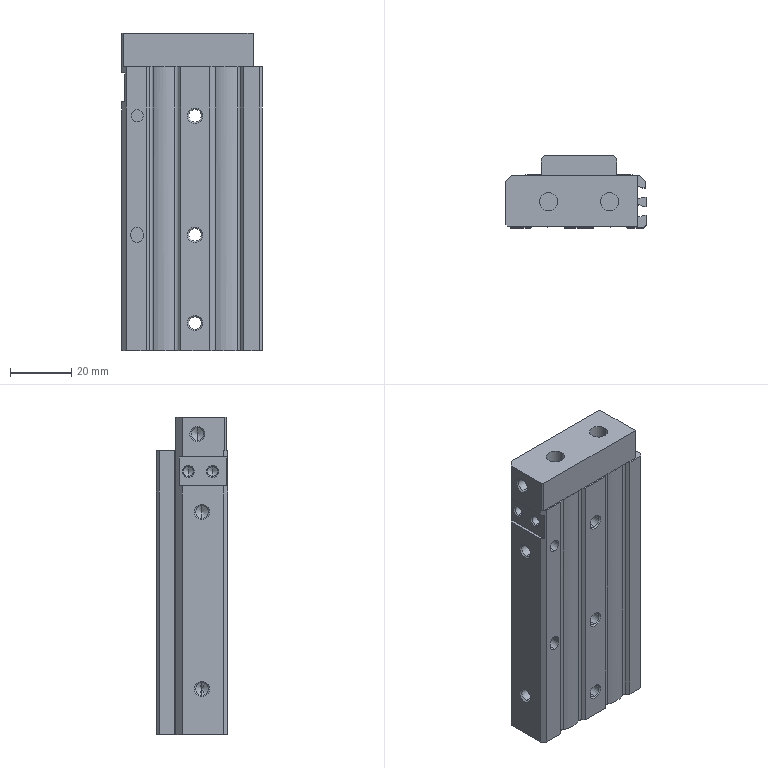Part | SolidWorks | features RefAxis 21, 3DProfileFeature 7, ICE 7, HoleWzd 6, LPattern 5, RevCut 5, Extrusion 1 | 1 solid | 165 faces | box 46 x 23.5 x 104 mm | volume 75785 mm3 | plane 66 | cylinder 57 | cone 42 | commonest cylinder face diameters 3.242 x12 4.134 x12 4 x9 8.5 x6 2 x4 6 x4